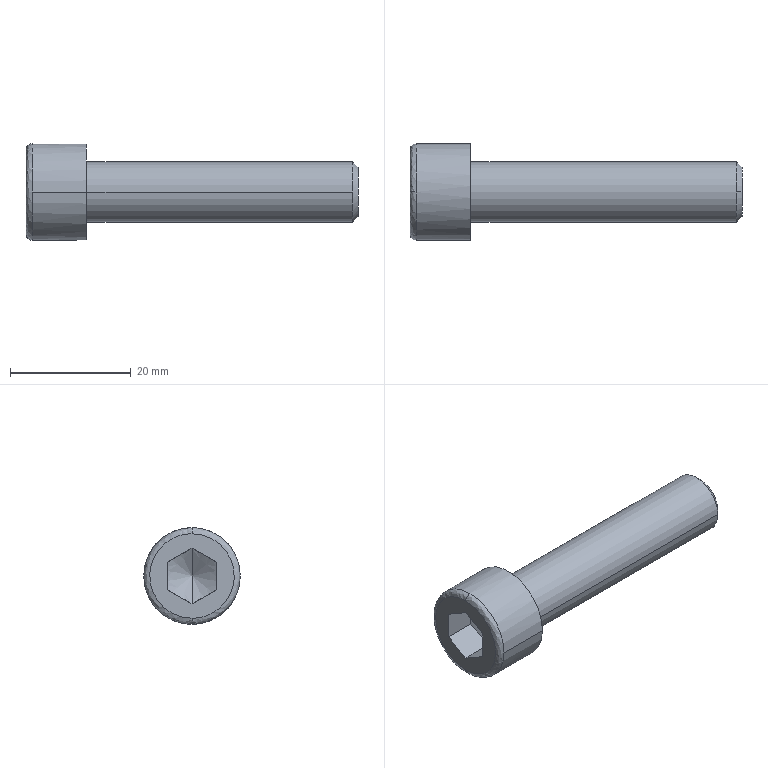Part | STEP file | AS 1420 - Metric M10 x 45 | 1 solid | 21 faces | box 55 x 16 x 16 mm | volume 5187 mm3 | plane 9 | spline 4 | cylinder 4 | cone 4 | commonest cylinder face diameters 10 x2 16 x2